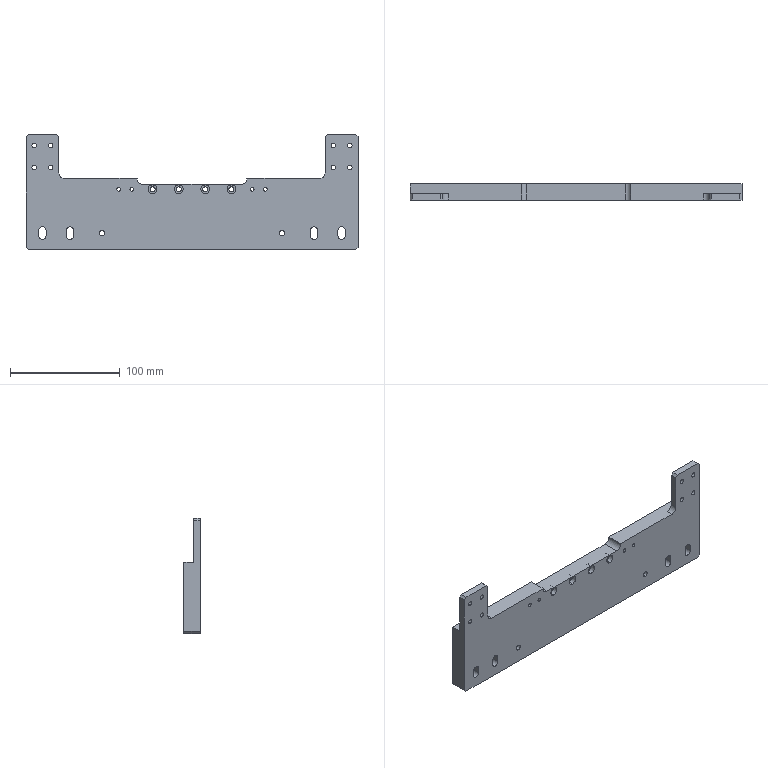Part | SolidWorks | features BaseBody 1 | 1 solid | 118 faces | box 303 x 15 x 105 mm | volume 292213 mm3 | cylinder 72 | plane 46 | commonest cylinder face diameters 4.2 x16 6.6 x12 11 x12 3.3 x8 4.5 x8 8 x8